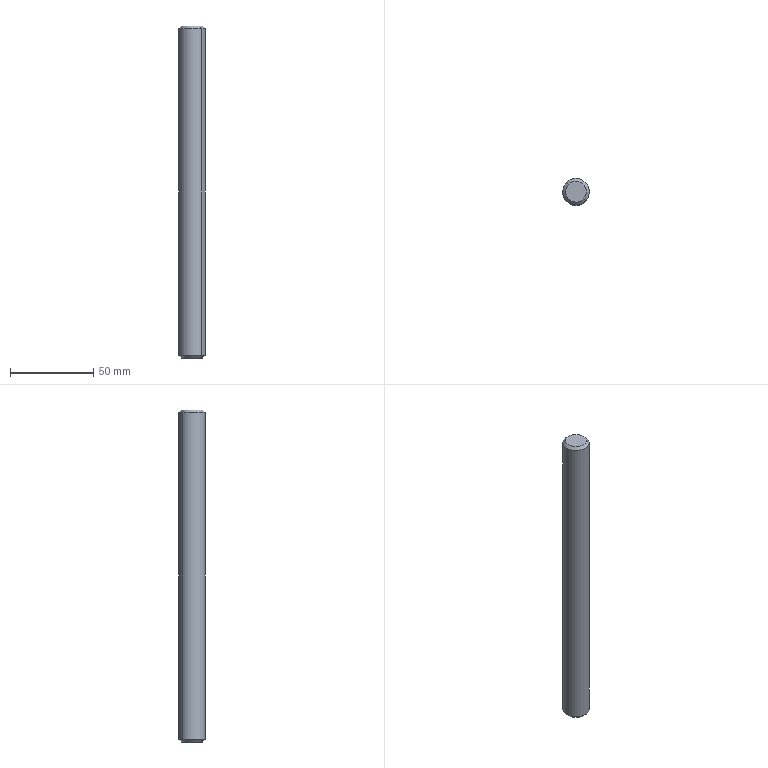Part | STEP file | Input 131 | 1 solid | 8 faces | box 16 x 16 x 200 mm | volume 40070 mm3 | cone 4 | cylinder 2 | plane 2 | commonest cylinder face diameters 16 x2
STEP:
#1=CARTESIAN_POINT('',(0.,0.,0.));
#2=DIRECTION('',(0.,0.,1.));
#3=DIRECTION('',(1.,0.,0.));
#4=AXIS2_PLACEMENT_3D('',#1,#2,#3);
#5=CARTESIAN_POINT('',(305.499,4.337,-252.));
#6=VERTEX_POINT('',#5);
#7=CARTESIAN_POINT('',(314.501,-4.337,-252.));
#8=VERTEX_POINT('',#7);
#9=CARTESIAN_POINT('',(310.,0.,-252.));
#10=DIRECTION('',(0.,0.,1.));
#11=DIRECTION('',(-0.7201,0.6939,0.));
#12=AXIS2_PLACEMENT_3D('',#9,#10,#11);
#13=CIRCLE('',#12,6.25);
#14=CARTESIAN_POINT('',(310.,0.,-250.25));
#15=DIRECTION('',(0.,0.,1.));
#16=DIRECTION('',(-0.7201,0.6939,0.));
#17=AXIS2_PLACEMENT_3D('',#14,#15,#16);
#18=CONICAL_SURFACE('',#17,8.,0.7854);
#19=CARTESIAN_POINT('',(0.,-1.75));
#20=DIRECTION('',(1.,0.));
#21=VECTOR('',#20,1.);
#22=LINE('',#19,#21);
#23=(GEOMETRIC_REPRESENTATION_CONTEXT(2)PARAMETRIC_REPRESENTATION_CONTEXT()REPRESENTATION_CONTEXT('',''));
#24=DEFINITIONAL_REPRESENTATION('',(#22),#23);
#25=PCURVE('',#18,#24);
#26=CARTESIAN_POINT('',(310.,0.,-252.));
#27=DIRECTION('',(0.,0.,-1.));
#28=DIRECTION('',(0.7201,-0.6939,0.));
#29=AXIS2_PLACEMENT_3D('',#26,#27,#28);
#30=PLANE('',#29);
#31=CARTESIAN_POINT('',(-6.25,0.));
#32=CARTESIAN_POINT('',(-6.25,10.825));
#33=CARTESIAN_POINT('',(3.125,5.413));
#34=CARTESIAN_POINT('',(12.5,0.));
#35=CARTESIAN_POINT('',(3.125,-5.413));
#36=CARTESIAN_POINT('',(-6.25,-10.825));
#37=CARTESIAN_POINT('',(-6.25,0.));
#38=(BOUNDED_CURVE()B_SPLINE_CURVE(2,(#31,#32,#33,#34,#35,#36,#37),.UNSPECIFIED.,.T.,.F.)B_SPLINE_CURVE_WITH_KNOTS((1,2,2,2,2,1),(-2.094,0.,2.094,4.189,6.283,8.378),.UNSPECIFIED.)CURVE()GEOMETRIC_REPRESENTATION_ITEM()RATIONAL_B_SPLINE_CURVE((1.,0.5,1.,0.5,1.,0.5,1.))REPRESENTATION_ITEM(''));
#39=(GEOMETRIC_REPRESENTATION_CONTEXT(2)PARAMETRIC_REPRESENTATION_CONTEXT()REPRESENTATION_CONTEXT('',''));
#40=DEFINITIONAL_REPRESENTATION('',(#38),#39);
#41=PCURVE('',#30,#40);
#42=SURFACE_CURVE('',#13,(#25,#41),.PCURVE_S1.);
#43=EDGE_CURVE('',#6,#8,#42,.T.);
#44=ORIENTED_EDGE('',*,*,#43,.T.);
#45=CARTESIAN_POINT('',(315.761,-5.551,-250.25));
#46=VERTEX_POINT('',#45);
#47=CARTESIAN_POINT('',(315.761,-5.551,-250.25));
#48=DIRECTION('',(0.5092,-0.4907,0.7071));
#49=VECTOR('',#48,1.);
#50=LINE('',#47,#49);
#51=CARTESIAN_POINT('',(3.142,0.));
#52=DIRECTION('',(0.,1.));
#53=VECTOR('',#52,1.);
#54=LINE('',#51,#53);
#55=(GEOMETRIC_REPRESENTATION_CONTEXT(2)PARAMETRIC_REPRESENTATION_CONTEXT()REPRESENTATION_CONTEXT('',''));
#56=DEFINITIONAL_REPRESENTATION('',(#54),#55);
#57=PCURVE('',#18,#56);
#58=CARTESIAN_POINT('',(310.,0.,-250.25));
#59=DIRECTION('',(0.,0.,1.));
#60=DIRECTION('',(-0.7201,0.6939,0.));
#61=AXIS2_PLACEMENT_3D('',#58,#59,#60);
#62=CONICAL_SURFACE('',#61,8.,0.7854);
#63=CARTESIAN_POINT('',(3.142,0.));
#64=DIRECTION('',(0.,1.));
#65=VECTOR('',#64,1.);
#66=LINE('',#63,#65);
#67=(GEOMETRIC_REPRESENTATION_CONTEXT(2)PARAMETRIC_REPRESENTATION_CONTEXT()REPRESENTATION_CONTEXT('',''));
#68=DEFINITIONAL_REPRESENTATION('',(#66),#67);
#69=PCURVE('',#62,#68);
#70=SURFACE_CURVE('',#50,(#57,#69),.PCURVE_S1.);
#71=EDGE_CURVE('',#8,#46,#70,.T.);
#72=ORIENTED_EDGE('',*,*,#71,.T.);
#73=CARTESIAN_POINT('',(304.239,5.551,-250.25));
#74=VERTEX_POINT('',#73);
#75=CARTESIAN_POINT('',(310.,0.,-250.25));
#76=DIRECTION('',(0.,0.,1.));
#77=DIRECTION('',(-0.7201,0.6939,0.));
#78=AXIS2_PLACEMENT_3D('',#75,#76,#77);
#79=CIRCLE('',#78,8.);
#80=CARTESIAN_POINT('',(0.,0.));
#81=DIRECTION('',(1.,0.));
#82=VECTOR('',#81,1.);
#83=LINE('',#80,#82);
#84=(GEOMETRIC_REPRESENTATION_CONTEXT(2)PARAMETRIC_REPRESENTATION_CONTEXT()REPRESENTATION_CONTEXT('',''));
#85=DEFINITIONAL_REPRESENTATION('',(#83),#84);
#86=PCURVE('',#18,#85);
#87=CARTESIAN_POINT('',(310.,0.,-52.));
#88=DIRECTION('',(0.,0.,1.));
#89=DIRECTION('',(-0.7201,0.6939,0.));
#90=AXIS2_PLACEMENT_3D('',#87,#88,#89);
#91=CYLINDRICAL_SURFACE('',#90,8.);
#92=CARTESIAN_POINT('',(0.,-198.25));
#93=DIRECTION('',(1.,0.));
#94=VECTOR('',#93,1.);
#95=LINE('',#92,#94);
#96=(GEOMETRIC_REPRESENTATION_CONTEXT(2)PARAMETRIC_REPRESENTATION_CONTEXT()REPRESENTATION_CONTEXT('',''));
#97=DEFINITIONAL_REPRESENTATION('',(#95),#96);
#98=PCURVE('',#91,#97);
#99=SURFACE_CURVE('',#79,(#86,#98),.PCURVE_S1.);
#100=EDGE_CURVE('',#74,#46,#99,.T.);
#101=ORIENTED_EDGE('',*,*,#100,.F.);
#102=CARTESIAN_POINT('',(304.239,5.551,-250.25));
#103=DIRECTION('',(-0.5092,0.4907,0.7071));
#104=VECTOR('',#103,1.);
#105=LINE('',#102,#104);
#106=CARTESIAN_POINT('',(0.,0.));
#107=DIRECTION('',(0.,1.));
#108=VECTOR('',#107,1.);
#109=LINE('',#106,#108);
#110=(GEOMETRIC_REPRESENTATION_CONTEXT(2)PARAMETRIC_REPRESENTATION_CONTEXT()REPRESENTATION_CONTEXT('',''));
#111=DEFINITIONAL_REPRESENTATION('',(#109),#110);
#112=PCURVE('',#18,#111);
#113=CARTESIAN_POINT('',(6.283,0.));
#114=DIRECTION('',(0.,1.));
#115=VECTOR('',#114,1.);
#116=LINE('',#113,#115);
#117=(GEOMETRIC_REPRESENTATION_CONTEXT(2)PARAMETRIC_REPRESENTATION_CONTEXT()REPRESENTATION_CONTEXT('',''));
#118=DEFINITIONAL_REPRESENTATION('',(#116),#117);
#119=PCURVE('',#62,#118);
#120=SURFACE_CURVE('',#105,(#112,#119),.PCURVE_S1.);
#121=EDGE_CURVE('',#6,#74,#120,.T.);
#122=ORIENTED_EDGE('',*,*,#121,.F.);
#123=EDGE_LOOP('',(#44,#72,#101,#122));
#124=FACE_BOUND('',#123,.T.);
#125=ADVANCED_FACE('',(#124),#18,.T.);
#126=ORIENTED_EDGE('',*,*,#100,.T.);
#127=CARTESIAN_POINT('',(315.761,-5.551,-53.75));
#128=VERTEX_POINT('',#127);
#129=CARTESIAN_POINT('',(315.761,-5.551,-52.));
#130=DIRECTION('',(0.,0.,1.));
#131=VECTOR('',#130,1.);
#132=LINE('',#129,#131);
#133=CARTESIAN_POINT('',(3.142,0.));
#134=DIRECTION('',(0.,1.));
#135=VECTOR('',#134,1.);
#136=LINE('',#133,#135);
#137=(GEOMETRIC_REPRESENTATION_CONTEXT(2)PARAMETRIC_REPRESENTATION_CONTEXT()REPRESENTATION_CONTEXT('',''));
#138=DEFINITIONAL_REPRESENTATION('',(#136),#137);
#139=PCURVE('',#91,#138);
#140=CARTESIAN_POINT('',(310.,0.,-52.));
#141=DIRECTION('',(0.,0.,1.));
#142=DIRECTION('',(-0.7201,0.6939,0.));
#143=AXIS2_PLACEMENT_3D('',#140,#141,#142);
#144=CYLINDRICAL_SURFACE('',#143,8.);
#145=CARTESIAN_POINT('',(3.142,0.));
#146=DIRECTION('',(0.,1.));
#147=VECTOR('',#146,1.);
#148=LINE('',#145,#147);
#149=(GEOMETRIC_REPRESENTATION_CONTEXT(2)PARAMETRIC_REPRESENTATION_CONTEXT()REPRESENTATION_CONTEXT('',''));
#150=DEFINITIONAL_REPRESENTATION('',(#148),#149);
#151=PCURVE('',#144,#150);
#152=SURFACE_CURVE('',#132,(#139,#151),.PCURVE_S1.);
#153=EDGE_CURVE('',#46,#128,#152,.T.);
#154=ORIENTED_EDGE('',*,*,#153,.T.);
#155=CARTESIAN_POINT('',(304.239,5.551,-53.75));
#156=VERTEX_POINT('',#155);
#157=CARTESIAN_POINT('',(310.,0.,-53.75));
#158=DIRECTION('',(0.,0.,1.));
#159=DIRECTION('',(-0.7201,0.6939,0.));
#160=AXIS2_PLACEMENT_3D('',#157,#158,#159);
#161=CIRCLE('',#160,8.);
#162=CARTESIAN_POINT('',(0.,-1.75));
#163=DIRECTION('',(1.,0.));
#164=VECTOR('',#163,1.);
#165=LINE('',#162,#164);
#166=(GEOMETRIC_REPRESENTATION_CONTEXT(2)PARAMETRIC_REPRESENTATION_CONTEXT()REPRESENTATION_CONTEXT('',''));
#167=DEFINITIONAL_REPRESENTATION('',(#165),#166);
#168=PCURVE('',#91,#167);
#169=CARTESIAN_POINT('',(310.,0.,-52.));
#170=DIRECTION('',(0.,0.,-1.));
#171=DIRECTION('',(0.7201,-0.6939,0.));
#172=AXIS2_PLACEMENT_3D('',#169,#170,#171);
#173=CONICAL_SURFACE('',#172,6.25,0.7854);
#174=CARTESIAN_POINT('',(3.142,1.75));
#175=DIRECTION('',(-1.,0.));
#176=VECTOR('',#175,1.);
#177=LINE('',#174,#176);
#178=(GEOMETRIC_REPRESENTATION_CONTEXT(2)PARAMETRIC_REPRESENTATION_CONTEXT()REPRESENTATION_CONTEXT('',''));
#179=DEFINITIONAL_REPRESENTATION('',(#177),#178);
#180=PCURVE('',#173,#179);
#181=SURFACE_CURVE('',#161,(#168,#180),.PCURVE_S1.);
#182=EDGE_CURVE('',#156,#128,#181,.T.);
#183=ORIENTED_EDGE('',*,*,#182,.F.);
#184=CARTESIAN_POINT('',(304.239,5.551,-52.));
#185=DIRECTION('',(0.,0.,1.));
#186=VECTOR('',#185,1.);
#187=LINE('',#184,#186);
#188=CARTESIAN_POINT('',(0.,0.));
#189=DIRECTION('',(0.,1.));
#190=VECTOR('',#189,1.);
#191=LINE('',#188,#190);
#192=(GEOMETRIC_REPRESENTATION_CONTEXT(2)PARAMETRIC_REPRESENTATION_CONTEXT()REPRESENTATION_CONTEXT('',''));
#193=DEFINITIONAL_REPRESENTATION('',(#191),#192);
#194=PCURVE('',#91,#193);
#195=CARTESIAN_POINT('',(6.283,0.));
#196=DIRECTION('',(0.,1.));
#197=VECTOR('',#196,1.);
#198=LINE('',#195,#197);
#199=(GEOMETRIC_REPRESENTATION_CONTEXT(2)PARAMETRIC_REPRESENTATION_CONTEXT()REPRESENTATION_CONTEXT('',''));
#200=DEFINITIONAL_REPRESENTATION('',(#198),#199);
#201=PCURVE('',#144,#200);
#202=SURFACE_CURVE('',#187,(#194,#201),.PCURVE_S1.);
#203=EDGE_CURVE('',#74,#156,#202,.T.);
#204=ORIENTED_EDGE('',*,*,#203,.F.);
#205=EDGE_LOOP('',(#126,#154,#183,#204));
#206=FACE_BOUND('',#205,.T.);
#207=ADVANCED_FACE('',(#206),#91,.T.);
#208=CARTESIAN_POINT('',(305.499,4.337,-52.));
#209=VERTEX_POINT('',#208);
#210=CARTESIAN_POINT('',(314.501,-4.337,-52.));
#211=VERTEX_POINT('',#210);
#212=CARTESIAN_POINT('',(310.,0.,-52.));
#213=DIRECTION('',(0.,0.,1.));
#214=DIRECTION('',(-0.7201,0.6939,0.));
#215=AXIS2_PLACEMENT_3D('',#212,#213,#214);
#216=CIRCLE('',#215,6.25);
#217=CARTESIAN_POINT('',(3.142,0.));
#218=DIRECTION('',(-1.,0.));
#219=VECTOR('',#218,1.);
#220=LINE('',#217,#219);
#221=(GEOMETRIC_REPRESENTATION_CONTEXT(2)PARAMETRIC_REPRESENTATION_CONTEXT()REPRESENTATION_CONTEXT('',''));
#222=DEFINITIONAL_REPRESENTATION('',(#220),#221);
#223=PCURVE('',#173,#222);
#224=CARTESIAN_POINT('',(310.,0.,-52.));
#225=DIRECTION('',(0.,0.,1.));
#226=DIRECTION('',(-0.7201,0.6939,0.));
#227=AXIS2_PLACEMENT_3D('',#224,#225,#226);
#228=PLANE('',#227);
#229=CARTESIAN_POINT('',(0.,0.));
#230=DIRECTION('',(1.,0.));
#231=AXIS2_PLACEMENT_2D('',#229,#230);
#232=CIRCLE('',#231,6.25);
#233=(GEOMETRIC_REPRESENTATION_CONTEXT(2)PARAMETRIC_REPRESENTATION_CONTEXT()REPRESENTATION_CONTEXT('',''));
#234=DEFINITIONAL_REPRESENTATION('',(#232),#233);
#235=PCURVE('',#228,#234);
#236=SURFACE_CURVE('',#216,(#223,#235),.PCURVE_S1.);
#237=EDGE_CURVE('',#209,#211,#236,.T.);
#238=ORIENTED_EDGE('',*,*,#237,.F.);
#239=CARTESIAN_POINT('',(305.499,4.337,-52.));
#240=DIRECTION('',(-0.5092,0.4907,-0.7071));
#241=VECTOR('',#240,1.);
#242=LINE('',#239,#241);
#243=CARTESIAN_POINT('',(3.142,0.));
#244=DIRECTION('',(0.,1.));
#245=VECTOR('',#244,1.);
#246=LINE('',#243,#245);
#247=(GEOMETRIC_REPRESENTATION_CONTEXT(2)PARAMETRIC_REPRESENTATION_CONTEXT()REPRESENTATION_CONTEXT('',''));
#248=DEFINITIONAL_REPRESENTATION('',(#246),#247);
#249=PCURVE('',#173,#248);
#250=CARTESIAN_POINT('',(310.,0.,-52.));
#251=DIRECTION('',(0.,0.,-1.));
#252=DIRECTION('',(0.7201,-0.6939,0.));
#253=AXIS2_PLACEMENT_3D('',#250,#251,#252);
#254=CONICAL_SURFACE('',#253,6.25,0.7854);
#255=CARTESIAN_POINT('',(3.142,0.));
#256=DIRECTION('',(0.,1.));
#257=VECTOR('',#256,1.);
#258=LINE('',#255,#257);
#259=(GEOMETRIC_REPRESENTATION_CONTEXT(2)PARAMETRIC_REPRESENTATION_CONTEXT()REPRESENTATION_CONTEXT('',''));
#260=DEFINITIONAL_REPRESENTATION('',(#258),#259);
#261=PCURVE('',#254,#260);
#262=SURFACE_CURVE('',#242,(#249,#261),.PCURVE_S1.);
#263=EDGE_CURVE('',#209,#156,#262,.T.);
#264=ORIENTED_EDGE('',*,*,#263,.T.);
#265=ORIENTED_EDGE('',*,*,#182,.T.);
#266=CARTESIAN_POINT('',(314.501,-4.337,-52.));
#267=DIRECTION('',(0.5092,-0.4907,-0.7071));
#268=VECTOR('',#267,1.);
#269=LINE('',#266,#268);
#270=CARTESIAN_POINT('',(0.,0.));
#271=DIRECTION('',(0.,1.));
#272=VECTOR('',#271,1.);
#273=LINE('',#270,#272);
#274=(GEOMETRIC_REPRESENTATION_CONTEXT(2)PARAMETRIC_REPRESENTATION_CONTEXT()REPRESENTATION_CONTEXT('',''));
#275=DEFINITIONAL_REPRESENTATION('',(#273),#274);
#276=PCURVE('',#173,#275);
#277=CARTESIAN_POINT('',(6.283,0.));
#278=DIRECTION('',(0.,1.));
#279=VECTOR('',#278,1.);
#280=LINE('',#277,#279);
#281=(GEOMETRIC_REPRESENTATION_CONTEXT(2)PARAMETRIC_REPRESENTATION_CONTEXT()REPRESENTATION_CONTEXT('',''));
#282=DEFINITIONAL_REPRESENTATION('',(#280),#281);
#283=PCURVE('',#254,#282);
#284=SURFACE_CURVE('',#269,(#276,#283),.PCURVE_S1.);
#285=EDGE_CURVE('',#211,#128,#284,.T.);
#286=ORIENTED_EDGE('',*,*,#285,.F.);
#287=EDGE_LOOP('',(#238,#264,#265,#286));
#288=FACE_BOUND('',#287,.T.);
#289=ADVANCED_FACE('',(#288),#173,.T.);
#290=CARTESIAN_POINT('',(310.,0.,-52.));
#291=DIRECTION('',(0.,0.,1.));
#292=DIRECTION('',(-0.7201,0.6939,0.));
#293=AXIS2_PLACEMENT_3D('',#290,#291,#292);
#294=CIRCLE('',#293,6.25);
#295=CARTESIAN_POINT('',(0.,0.));
#296=DIRECTION('',(1.,0.));
#297=AXIS2_PLACEMENT_2D('',#295,#296);
#298=CIRCLE('',#297,6.25);
#299=(GEOMETRIC_REPRESENTATION_CONTEXT(2)PARAMETRIC_REPRESENTATION_CONTEXT()REPRESENTATION_CONTEXT('',''));
#300=DEFINITIONAL_REPRESENTATION('',(#298),#299);
#301=PCURVE('',#228,#300);
#302=CARTESIAN_POINT('',(9.425,0.));
#303=DIRECTION('',(-1.,0.));
#304=VECTOR('',#303,1.);
#305=LINE('',#302,#304);
#306=(GEOMETRIC_REPRESENTATION_CONTEXT(2)PARAMETRIC_REPRESENTATION_CONTEXT()REPRESENTATION_CONTEXT('',''));
#307=DEFINITIONAL_REPRESENTATION('',(#305),#306);
#308=PCURVE('',#254,#307);
#309=SURFACE_CURVE('',#294,(#301,#308),.PCURVE_S1.);
#310=EDGE_CURVE('',#211,#209,#309,.T.);
#311=ORIENTED_EDGE('',*,*,#310,.T.);
#312=ORIENTED_EDGE('',*,*,#237,.T.);
#313=EDGE_LOOP('',(#311,#312));
#314=FACE_BOUND('',#313,.T.);
#315=ADVANCED_FACE('',(#314),#228,.T.);
#316=ORIENTED_EDGE('',*,*,#263,.F.);
#317=ORIENTED_EDGE('',*,*,#310,.F.);
#318=ORIENTED_EDGE('',*,*,#285,.T.);
#319=CARTESIAN_POINT('',(310.,0.,-53.75));
#320=DIRECTION('',(0.,0.,1.));
#321=DIRECTION('',(-0.7201,0.6939,0.));
#322=AXIS2_PLACEMENT_3D('',#319,#320,#321);
#323=CIRCLE('',#322,8.);
#324=CARTESIAN_POINT('',(9.425,1.75));
#325=DIRECTION('',(-1.,0.));
#326=VECTOR('',#325,1.);
#327=LINE('',#324,#326);
#328=(GEOMETRIC_REPRESENTATION_CONTEXT(2)PARAMETRIC_REPRESENTATION_CONTEXT()REPRESENTATION_CONTEXT('',''));
#329=DEFINITIONAL_REPRESENTATION('',(#327),#328);
#330=PCURVE('',#254,#329);
#331=CARTESIAN_POINT('',(0.,-1.75));
#332=DIRECTION('',(1.,0.));
#333=VECTOR('',#332,1.);
#334=LINE('',#331,#333);
#335=(GEOMETRIC_REPRESENTATION_CONTEXT(2)PARAMETRIC_REPRESENTATION_CONTEXT()REPRESENTATION_CONTEXT('',''));
#336=DEFINITIONAL_REPRESENTATION('',(#334),#335);
#337=PCURVE('',#144,#336);
#338=SURFACE_CURVE('',#323,(#330,#337),.PCURVE_S1.);
#339=EDGE_CURVE('',#128,#156,#338,.T.);
#340=ORIENTED_EDGE('',*,*,#339,.T.);
#341=EDGE_LOOP('',(#316,#317,#318,#340));
#342=FACE_BOUND('',#341,.T.);
#343=ADVANCED_FACE('',(#342),#254,.T.);
#344=ORIENTED_EDGE('',*,*,#153,.F.);
#345=CARTESIAN_POINT('',(310.,0.,-250.25));
#346=DIRECTION('',(0.,0.,1.));
#347=DIRECTION('',(-0.7201,0.6939,0.));
#348=AXIS2_PLACEMENT_3D('',#345,#346,#347);
#349=CIRCLE('',#348,8.);
#350=CARTESIAN_POINT('',(0.,-198.25));
#351=DIRECTION('',(1.,0.));
#352=VECTOR('',#351,1.);
#353=LINE('',#350,#352);
#354=(GEOMETRIC_REPRESENTATION_CONTEXT(2)PARAMETRIC_REPRESENTATION_CONTEXT()REPRESENTATION_CONTEXT('',''));
#355=DEFINITIONAL_REPRESENTATION('',(#353),#354);
#356=PCURVE('',#144,#355);
#357=CARTESIAN_POINT('',(0.,0.));
#358=DIRECTION('',(1.,0.));
#359=VECTOR('',#358,1.);
#360=LINE('',#357,#359);
#361=(GEOMETRIC_REPRESENTATION_CONTEXT(2)PARAMETRIC_REPRESENTATION_CONTEXT()REPRESENTATION_CONTEXT('',''));
#362=DEFINITIONAL_REPRESENTATION('',(#360),#361);
#363=PCURVE('',#62,#362);
#364=SURFACE_CURVE('',#349,(#356,#363),.PCURVE_S1.);
#365=EDGE_CURVE('',#46,#74,#364,.T.);
#366=ORIENTED_EDGE('',*,*,#365,.T.);
#367=ORIENTED_EDGE('',*,*,#203,.T.);
#368=ORIENTED_EDGE('',*,*,#339,.F.);
#369=EDGE_LOOP('',(#344,#366,#367,#368));
#370=FACE_BOUND('',#369,.T.);
#371=ADVANCED_FACE('',(#370),#144,.T.);
#372=ORIENTED_EDGE('',*,*,#71,.F.);
#373=CARTESIAN_POINT('',(310.,0.,-252.));
#374=DIRECTION('',(0.,0.,1.));
#375=DIRECTION('',(-0.7201,0.6939,0.));
#376=AXIS2_PLACEMENT_3D('',#373,#374,#375);
#377=CIRCLE('',#376,6.25);
#378=CARTESIAN_POINT('',(0.,-1.75));
#379=DIRECTION('',(1.,0.));
#380=VECTOR('',#379,1.);
#381=LINE('',#378,#380);
#382=(GEOMETRIC_REPRESENTATION_CONTEXT(2)PARAMETRIC_REPRESENTATION_CONTEXT()REPRESENTATION_CONTEXT('',''));
#383=DEFINITIONAL_REPRESENTATION('',(#381),#382);
#384=PCURVE('',#62,#383);
#385=CARTESIAN_POINT('',(-6.25,0.));
#386=CARTESIAN_POINT('',(-6.25,10.825));
#387=CARTESIAN_POINT('',(3.125,5.413));
#388=CARTESIAN_POINT('',(12.5,0.));
#389=CARTESIAN_POINT('',(3.125,-5.413));
#390=CARTESIAN_POINT('',(-6.25,-10.825));
#391=CARTESIAN_POINT('',(-6.25,0.));
#392=(BOUNDED_CURVE()B_SPLINE_CURVE(2,(#385,#386,#387,#388,#389,#390,#391),.UNSPECIFIED.,.T.,.F.)B_SPLINE_CURVE_WITH_KNOTS((1,2,2,2,2,1),(-2.094,0.,2.094,4.189,6.283,8.378),.UNSPECIFIED.)CURVE()GEOMETRIC_REPRESENTATION_ITEM()RATIONAL_B_SPLINE_CURVE((1.,0.5,1.,0.5,1.,0.5,1.))REPRESENTATION_ITEM(''));
#393=(GEOMETRIC_REPRESENTATION_CONTEXT(2)PARAMETRIC_REPRESENTATION_CONTEXT()REPRESENTATION_CONTEXT('',''));
#394=DEFINITIONAL_REPRESENTATION('',(#392),#393);
#395=PCURVE('',#30,#394);
#396=SURFACE_CURVE('',#377,(#384,#395),.PCURVE_S1.);
#397=EDGE_CURVE('',#8,#6,#396,.T.);
#398=ORIENTED_EDGE('',*,*,#397,.T.);
#399=ORIENTED_EDGE('',*,*,#121,.T.);
#400=ORIENTED_EDGE('',*,*,#365,.F.);
#401=EDGE_LOOP('',(#372,#398,#399,#400));
#402=FACE_BOUND('',#401,.T.);
#403=ADVANCED_FACE('',(#402),#62,.T.);
#404=ORIENTED_EDGE('',*,*,#43,.F.);
#405=ORIENTED_EDGE('',*,*,#397,.F.);
#406=EDGE_LOOP('',(#404,#405));
#407=FACE_BOUND('',#406,.T.);
#408=ADVANCED_FACE('',(#407),#30,.T.);
#409=CLOSED_SHELL('',(#125,#207,#289,#315,#343,#371,#403,#408));
#410=MANIFOLD_SOLID_BREP('',#409);
#411=(LENGTH_UNIT()NAMED_UNIT(*)SI_UNIT(.MILLI.,.METRE.));
#412=UNCERTAINTY_MEASURE_WITH_UNIT(LENGTH_MEASURE(0.0000001),#411,'','');
#413=(NAMED_UNIT(*)PLANE_ANGLE_UNIT()SI_UNIT($,.RADIAN.));
#414=(NAMED_UNIT(*)SI_UNIT($,.STERADIAN.)SOLID_ANGLE_UNIT());
#415=(GEOMETRIC_REPRESENTATION_CONTEXT(3)GLOBAL_UNCERTAINTY_ASSIGNED_CONTEXT((#412))GLOBAL_UNIT_ASSIGNED_CONTEXT((#411,#413,#414))REPRESENTATION_CONTEXT('',''));
#416=ADVANCED_BREP_SHAPE_REPRESENTATION('',(#4,#410),#415);